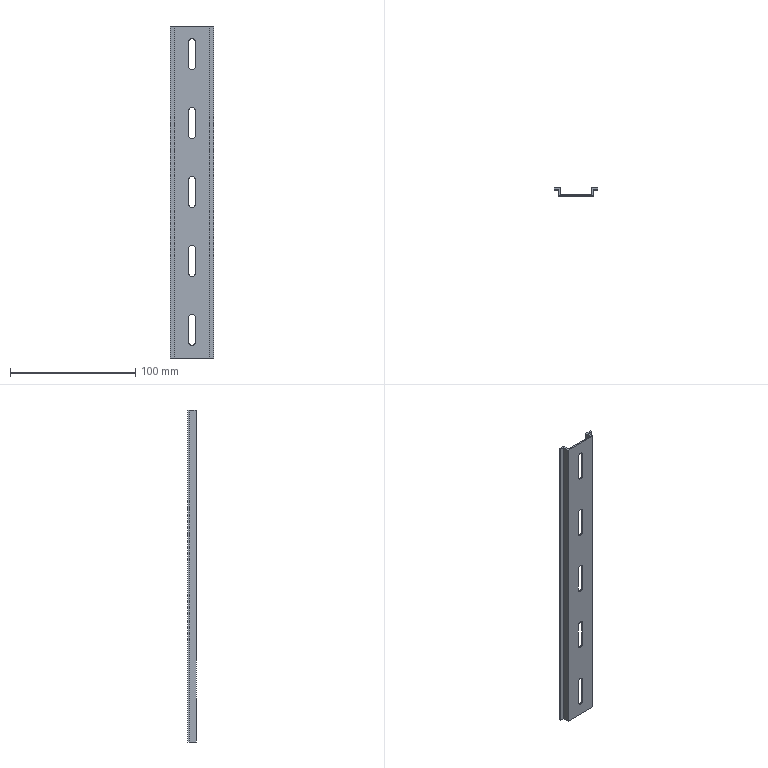Part | STEP file | card slot 35-265 | 1 solid | 34 faces | box 35 x 6.5 x 265 mm | volume 13977 mm3 | plane 24 | cylinder 10 | commonest cylinder face diameters 5 x10